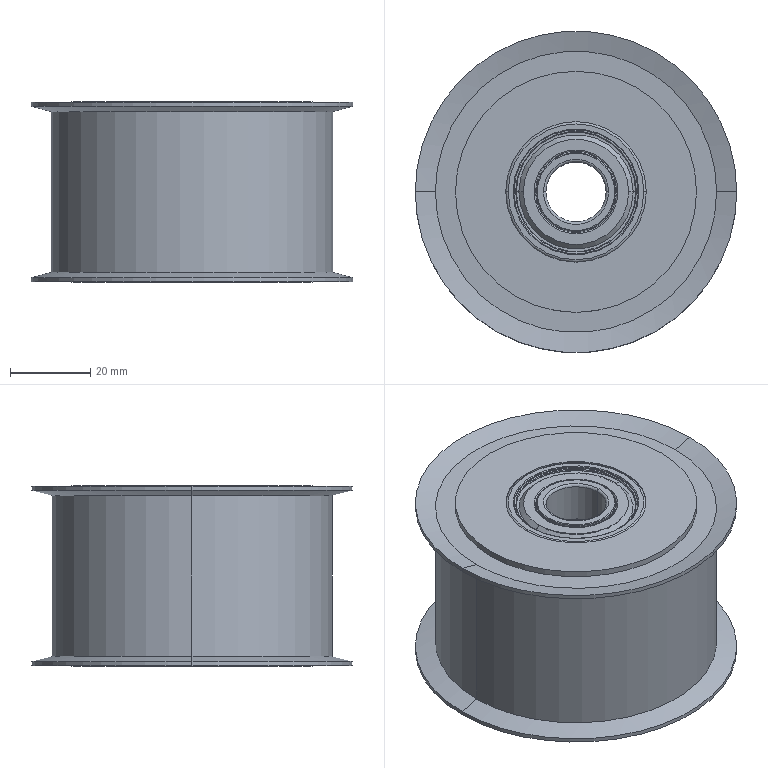Part | SolidWorks | features Revolution 3, LockFeature 1 | 1 solid | 278 faces | box 80 x 80 x 45 mm | volume 153277 mm3 | torus 88 | cylinder 80 | cone 80 | plane 30 | commonest cylinder face diameters 18.8 x8 19.7 x8 20.3 x8 20.9 x8 21.1 x8 28.9 x8